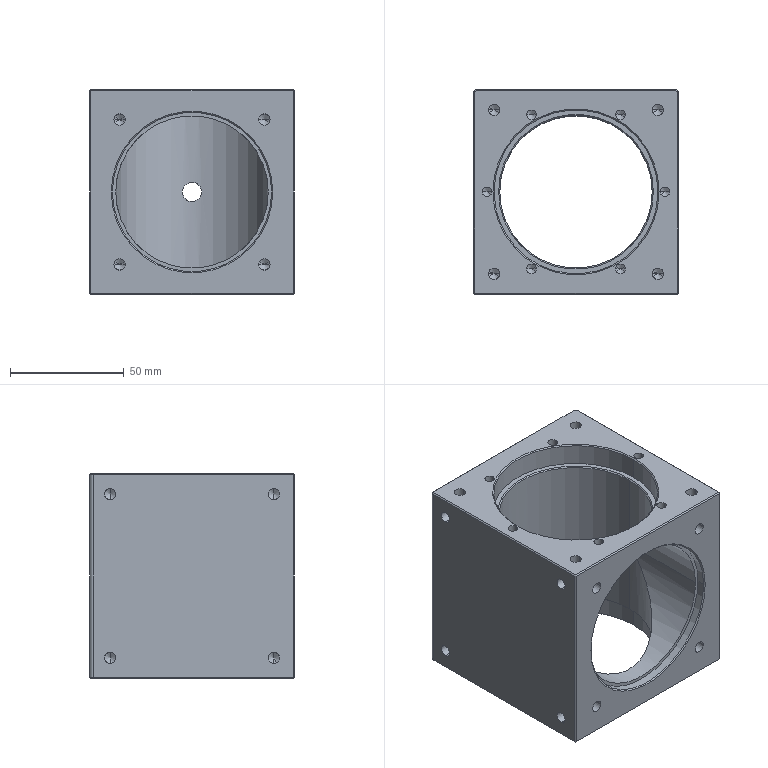NC program | NX | posted with a generic post | part box 90 x 90 x 90 mm
Whole program:
N10 G17 G21 G94 G90
(DRILLING_COPY_1_COPY_1_COPY , TOOL : D6A45)
N12 T07 M6
N14 G54
N16 G17 G0 G90 X19.55 Y-33.862 B0. C0. S5000 M3
N18 G43 Z30. H7
N20 G94 G81 G98 Z-1. F250. R3.
N22 X36. Y-36.
N24 X39.1 Y0.
N26 X36. Y36.
N28 X19.55 Y33.862
N30 X0. Y0.
N32 X-19.55 Y33.862
N34 X-36. Y36.
N36 X-39.1 Y0.
N38 X-36. Y-36.
N40 X-19.55 Y-33.862
N42 G80
N44 G0 X-19.55 Y-33.862 Z30.
N46 M5
(DRILLING_COPY_1_COPY_COPY_COPY_COPY_COPY_1 , TOOL : 5.0ZT)
N48 T15 M6
N50 G54
N52 G17 G0 G90 X36. Y-36. B0. C0. S2000 M3
N54 G43 Z30. H15
N56 G94 G83 G98 Z-12.002 F150. Q2. R3.
N58 X-36.
N60 Y36. Z-10.234
N62 X36.
N64 G80
N66 G0 X36. Y36. Z30.
N68 M5
(DRILLING_COPY_1_COPY_COPY_COPY_COPY_COPY_1_COPY , TOOL : 4.2ZT)
N70 T14 M6
N72 G54
N74 G17 G0 G90 X39.1 Y0. B0. C0. S2000 M3
N76 G43 Z30. H14
N78 G94 G83 G98 Z-15.262 F150. Q2. R3.
N80 X19.55 Y33.862
N82 X-19.55
N84 X-39.1 Y0.
N86 X-19.55 Y-33.862
N88 X19.55
N90 G80
N92 G0 X19.55 Y-33.862 Z30.
N94 M5
(DRILLING_COPY_1_COPY_COPY_COPY_COPY_COPY_COPY , TOOL : 9.0ZT)
N96 T09 M6
N98 G54
N100 G17 G0 G90 X0. Y0. B0. C0. S1200 M3
N102 G43 Z30. H9
N104 G94 G83 G98 Z-49.704 F150. Q2. R3.
N106 G80
N108 G0 X0. Y0. Z30.
N110 M5
(HOLE_MILLING_COPY_1 , TOOL : D10)
N112 T10 M6
N114 G54
N116 G17 G0 G90 X0. Y0. B0. C0. S9500 M3
N118 G43 Z30. H10
N120 Z0.5
N122 G94 G3 X1.25 Y-1.25 R1.25 F2200.
N124 X2.5 Y0. R1.25
N126 X2.5 Y0. Z-0.5 I-2.5 J0.
N128 X2.5 Y0. Z-1.5 I-2.5 J0.
N130 X2.5 Y0. Z-2.5 I-2.5 J0.
N132 X2.5 Y0. Z-3.5 I-2.5 J0.
N134 X2.5 Y0. Z-4.5 I-2.5 J0.
N136 X2.5 Y0. Z-5.5 I-2.5 J0.
N138 X2.5 Y0. Z-6.5 I-2.5 J0.
N140 X2.5 Y0. Z-7.5 I-2.5 J0.
N142 X2.5 Y0. Z-8.5 I-2.5 J0.
N144 X2.5 Y0. Z-9.5 I-2.5 J0.
N146 X-0.099 Y2.678 R2.68
N148 X-2.987 Y0.165 R2.819
N150 X-0.334 Y-3.217 R3.076
N152 X3.461 Y-0.383 R3.39
N154 X0.578 Y3.681 R3.568
N156 X-3.919 Y0.654 R3.881
N158 X-0.874 Y-4.126 R4.06
N160 X4.357 Y-0.976 R4.373
N162 X1.22 Y4.548 R4.551
N164 X-4.769 Y1.349 R4.865
N166 X-1.615 Y-4.943 R5.043
N168 X5.152 Y-1.769 R5.356
N170 X2.058 Y5.307 R5.534
N172 X-5.502 Y2.235 R5.847
N174 X-2.544 Y-5.635 R6.025
N176 X5.815 Y-2.744 R6.339
N178 X3.072 Y5.925 R6.517
N180 X-6.087 Y3.294 R6.83
N182 X-3.64 Y-6.172 R7.008
N184 X6.315 Y-3.882 R7.322
N186 X4.243 Y6.374 R7.5
N188 X-6.495 Y4.503 R7.813
N190 X-4.879 Y-6.526 R7.991
N192 X6.625 Y-5.156 R8.304
N194 X5.543 Y6.627 R8.482
N196 X-6.701 Y5.836 R8.796
N198 X-6.232 Y-6.673 R8.974
N200 X6.721 Y-6.539 R9.287
N202 X6.943 Y6.662 R9.465
N204 X-6.684 Y7.26 R9.778
N206 X-7.67 Y-6.592 R9.956
N208 X6.586 Y-7.997 R10.269
N210 X8.409 Y6.461 R10.447
N212 X-6.426 Y8.743 R10.761
N214 X-9.156 Y-6.268 R10.939
N216 X6.204 Y-9.495 R11.252
N218 X9.906 Y6.012 R11.43
N220 X-5.917 Y10.248 R11.743
N222 X-10.654 Y-5.691 R11.921
N224 X5.565 Y-10.997 R12.235
N226 X11.395 Y5.305 R12.413
N228 X-5.148 Y11.736 R12.726
N230 X-12.125 Y-4.854 R12.904
N232 X4.666 Y-12.462 R13.217
N234 X12.839 Y4.338 R13.395
N236 X-4.119 Y13.169 R13.708
N238 X-13.531 Y-3.758 R13.886
N240 X3.508 Y-13.852 R14.2
N242 X14.197 Y3.114 R14.378
N244 X-2.834 Y14.507 R14.691
N246 X-14.832 Y-2.408 R14.869
N248 X2.098 Y-15.127 R15.182
N250 X15.43 Y1.642 R15.36
N252 X-1.302 Y15.709 R15.673
N254 X-15.987 Y-0.816 R15.851
N256 X0.448 Y-16.248 R16.165
N258 X16.499 Y-0.066 R16.343
N260 X0.461 Y16.739 R16.656
N262 X-16.961 Y1.002 R16.834
N264 X-1.423 Y-17.178 R17.147
N266 X17.369 Y-1.989 R17.325
N268 X2.435 Y17.56 R17.638
N270 X-17.717 Y3.023 R17.816
N272 X-3.493 Y-17.881 R18.13
N274 X18.003 Y-4.102 R18.308
N276 X4.593 Y18.138 R18.621
N278 X-18.222 Y5.221 R18.799
N280 X-5.732 Y-18.326 R19.112
N282 X18.372 Y-6.377 R19.29
N284 X6.905 Y18.443 R19.603
N286 X-18.448 Y7.564 R19.781
N288 X-8.108 Y-18.484 R20.095
N290 X18.447 Y-8.778 R20.273
N292 X9.336 Y18.448 R20.586
N294 X-18.368 Y10.015 R20.764
N296 X-10.583 Y-18.331 R21.077
N298 X18.207 Y-11.269 R21.255
N300 X11.846 Y18.131 R21.568
N302 X-17.962 Y12.535 R21.746
N304 X-13.117 Y-17.847 R22.06
N306 X17.632 Y-13.807 R22.238
N308 X14.393 Y17.476 R22.551
N310 X-17.215 Y15.08 R22.729
N312 X-15.667 Y-17.018 R23.042
N314 X16.71 Y-16.348 R23.22
N316 X16.932 Y16.472 R23.533
N318 X-16.117 Y17.605 R23.711
N320 X-18.185 Y-15.837 R24.025
N322 X15.435 Y-18.845 R24.202
N324 X19.417 Y15.113 R24.516
N326 X-14.664 Y20.063 R24.694
N328 X-20.624 Y-14.3 R25.007
N330 X13.805 Y-21.251 R25.185
N332 X21.799 Y13.4 R25.498
N334 X-12.859 Y22.405 R25.676
N336 X-22.936 Y-12.412 R25.989
N338 X11.827 Y-23.518 R26.167
N340 X24.029 Y11.34 R26.481
N342 X-10.711 Y24.583 R26.659
N344 X-25.072 Y-10.183 R26.972
N346 X9.513 Y-25.596 R27.15
N348 X26.06 Y8.946 R27.463
N350 X-8.235 Y26.55 R27.641
N352 X-26.986 Y-7.631 R27.954
N354 X6.881 Y-27.44 R28.132
N356 X27.844 Y6.24 R28.446
N358 X-5.453 Y28.259 R28.624
N360 X-28.63 Y-4.778 R28.937
N362 X3.955 Y-29.003 R29.115
N364 X29.338 Y3.247 R29.428
N366 X-2.392 Y29.667 R29.606
N368 X-29.963 Y-1.653 R29.919
N370 X1.001 Y-30.316 R30.177
N372 X30.5 Y0. R30.328
N374 X0. Y30.5 R30.5
N376 X30.5 Y0. R-30.5
N378 X15.25 Y15.25 R15.25
N380 X0. Y0. R15.25
N382 G0 Z30.
N384 M5
(HOLE_MILLING_COPY_COPY_1 , TOOL : D16)
N386 T16 M6
N388 G54
N390 G17 G0 G90 X0. Y0. B0. C0. S8500 M3
N392 G43 Z30. H16
N394 Z-9.
N396 G94 G3 X1.5 Y-1.5 R1.5 F2200.
N398 X3. Y0. R1.5
N400 X3. Y0. Z-10. I-3. J0.
N402 X3. Y0. Z-11. I-3. J0.
N404 X3. Y0. Z-12. I-3. J0.
N406 X3. Y0. Z-13. I-3. J0.
N408 X3. Y0. Z-14. I-3. J0.
N410 X3. Y0. Z-15. I-3. J0.
N412 X3. Y0. Z-16. I-3. J0.
N414 X3. Y0. Z-17. I-3. J0.
N416 X3. Y0. Z-18. I-3. J0.
N418 X3. Y0. Z-19. I-3. J0.
N420 X3. Y0. Z-20. I-3. J0.
N422 X3. Y0. Z-21. I-3. J0.
N424 X3. Y0. Z-22. I-3. J0.
N426 X3. Y0. Z-23. I-3. J0.
N428 X3. Y0. Z-24. I-3. J0.
N430 X3. Y0. Z-25. I-3. J0.
N432 X3. Y0. Z-26. I-3. J0.
N434 X3. Y0. Z-27. I-3. J0.
N436 X0. Y-3. Z-27.75 R-3.
N438 X3.177 Y0.141 R3.177
N440 X0.073 Y3.496 R3.325
N442 X-3.738 Y0.186 R3.583
N444 X-0.167 Y-3.99 R3.9
N446 X4.23 Y-0.29 R4.08
N448 X0.282 Y4.481 R4.397
N450 X-4.718 Y0.415 R4.577
N452 X-0.417 Y-4.969 R4.894
N454 X5.203 Y-0.56 R5.074
N456 X0.573 Y5.453 R5.391
N458 X-5.684 Y0.726 R5.571
N460 X-0.749 Y-5.933 R5.888
N462 X6.16 Y-0.912 R6.068
N464 X0.946 Y6.407 R6.385
N466 X-6.63 Y1.119 R6.565
N468 X-1.163 Y-6.876 R6.881
N470 X7.094 Y-1.345 R7.062
N472 X1.4 Y7.338 R7.378
N474 X-7.551 Y1.592 R7.558
N476 X-1.656 Y-7.793 R7.875
N478 X8.001 Y-1.858 R8.055
N480 X1.933 Y8.24 R8.372
N482 X-8.443 Y2.143 R8.552
N484 X-2.228 Y-8.679 R8.868
N486 X8.876 Y-2.448 R9.049
N488 X2.543 Y9.108 R9.365
N490 X-9.3 Y2.772 R9.545
N492 X-2.877 Y-9.529 R9.862
N494 X9.714 Y-3.115 R10.042
N496 X3.229 Y9.939 R10.359
N498 X-10.117 Y3.476 R10.539
N500 X-3.6 Y-10.338 R10.855
N502 X10.509 Y-3.855 R11.036
N504 X3.989 Y10.726 R11.352
N506 X-10.89 Y4.253 R11.532
N508 X-4.395 Y-11.102 R11.849
N510 X11.259 Y-4.667 R12.029
N512 X4.819 Y11.465 R12.346
N514 X-11.614 Y5.099 R12.526
N516 X-5.26 Y-11.815 R12.842
N518 X11.956 Y-5.548 R13.022
N520 X5.718 Y12.152 R13.339
N522 X-12.285 Y6.014 R13.519
N524 X-6.192 Y-12.474 R13.836
N526 X12.599 Y-6.495 R14.016
N528 X6.682 Y12.782 R14.332
N530 X-12.898 Y6.992 R14.513
N532 X-7.188 Y-13.074 R14.829
N534 X13.181 Y-7.505 R15.009
N536 X7.708 Y13.351 R15.326
N538 X-13.449 Y8.032 R15.506
N540 X-8.244 Y-13.612 R15.822
N542 X13.7 Y-8.573 R16.003
N544 X8.793 Y13.855 R16.319
N546 X-13.934 Y9.129 R16.499
N548 X-9.356 Y-14.082 R16.816
N550 X14.15 Y-9.698 R16.996
N552 X9.932 Y14.291 R17.312
N554 X-14.349 Y10.28 R17.493
N556 X-10.521 Y-14.481 R17.809
N558 X14.529 Y-10.874 R17.989
N560 X11.123 Y14.653 R18.306
N562 X-14.691 Y11.481 R18.486
N564 X-11.736 Y-14.807 R18.803
N566 X14.833 Y-12.098 R18.983
N568 X12.36 Y14.94 R19.299
N570 X-14.956 Y12.727 R19.479
N572 X-12.994 Y-15.054 R19.796
N574 X15.059 Y-13.366 R19.976
N576 X13.639 Y15.148 R20.293
N578 X-15.141 Y14.014 R20.473
N580 X-14.293 Y-15.221 R20.789
N582 X15.203 Y-14.672 R20.97
N584 X14.956 Y15.273 R21.286
N586 X-15.243 Y15.338 R21.466
N588 X-15.628 Y-15.304 R21.783
N590 X15.262 Y-16.013 R21.963
N592 X16.307 Y15.313 R22.279
N594 X-15.26 Y16.695 R22.46
N596 X-16.993 Y-15.301 R22.776
N598 X15.235 Y-17.383 R22.956
N600 X17.686 Y15.266 R23.273
N602 X-15.189 Y18.078 R23.453
N604 X-18.384 Y-15.209 R23.769
N606 X15.119 Y-18.778 R23.95
N608 X19.088 Y15.129 R24.266
N610 X-15.027 Y19.483 R24.446
N612 X-19.796 Y-15.026 R24.763
N614 X15.149 Y-20.116 R25.023
N616 X20.509 Y14.9 R25.179
N618 X-14.9 Y20.509 R25.35
N620 X20.509 Y14.9 R-25.35
N622 X2.804 Y17.704 R12.675
N624 X0. Y0. R12.675
N626 X1.5 Y-1.5 R1.5
N628 X3. Y0. R1.5
N630 X3. Y0. Z-28.75 I-3. J0.
N632 X3. Y0. Z-29.75 I-3. J0.
N634 X3. Y0. Z-30.75 I-3. J0.
N636 X3. Y0. Z-31.75 I-3. J0.
N638 X3. Y0. Z-32.75 I-3. J0.
N640 X3. Y0. Z-33.75 I-3. J0.
N642 X3. Y0. Z-34.75 I-3. J0.
N644 X3. Y0. Z-35.75 I-3. J0.
N646 X3. Y0. Z-36.75 I-3. J0.
N648 X3. Y0. Z-37.75 I-3. J0.
N650 X3. Y0. Z-38.75 I-3. J0.
N652 X3. Y0. Z-39.75 I-3. J0.
N654 X3. Y0. Z-40.75 I-3. J0.
N656 X3. Y0. Z-41.75 I-3. J0.
N658 X3. Y0. Z-42.75 I-3. J0.
N660 X3. Y0. Z-43.75 I-3. J0.
N662 X3. Y0. Z-44.75 I-3. J0.
N664 X3. Y0. Z-45.75 I-3. J0.
N666 X0. Y-3. Z-46.5 R-3.
N668 X3.177 Y0.141 R3.177
N670 X0.073 Y3.496 R3.325
N672 X-3.738 Y0.186 R3.583
N674 X-0.167 Y-3.99 R3.9
N676 X4.23 Y-0.29 R4.08
N678 X0.282 Y4.481 R4.397
N680 X-4.718 Y0.415 R4.577
N682 X-0.417 Y-4.969 R4.894
N684 X5.203 Y-0.56 R5.074
N686 X0.573 Y5.453 R5.391
N688 X-5.684 Y0.726 R5.571
N690 X-0.749 Y-5.933 R5.888
N692 X6.16 Y-0.912 R6.068
N694 X0.946 Y6.407 R6.385
N696 X-6.63 Y1.119 R6.565
N698 X-1.163 Y-6.876 R6.881
N700 X7.094 Y-1.345 R7.062
N702 X1.4 Y7.338 R7.378
N704 X-7.551 Y1.592 R7.558
N706 X-1.656 Y-7.793 R7.875
N708 X8.001 Y-1.858 R8.055
N710 X1.933 Y8.24 R8.372
N712 X-8.443 Y2.143 R8.552
N714 X-2.228 Y-8.679 R8.868
N716 X8.876 Y-2.448 R9.049
N718 X2.543 Y9.108 R9.365
N720 X-9.3 Y2.772 R9.545
N722 X-2.877 Y-9.529 R9.862
N724 X9.714 Y-3.115 R10.042
N726 X3.229 Y9.939 R10.359
N728 X-10.117 Y3.476 R10.539
N730 X-3.6 Y-10.338 R10.855
N732 X10.509 Y-3.855 R11.036
N734 X3.989 Y10.726 R11.352
N736 X-10.89 Y4.253 R11.532
N738 X-4.395 Y-11.102 R11.849
N740 X11.259 Y-4.667 R12.029
N742 X4.819 Y11.465 R12.346
N744 X-11.614 Y5.099 R12.526
N746 X-5.26 Y-11.815 R12.842
N748 X11.956 Y-5.548 R13.022
N750 X5.718 Y12.152 R13.339
N752 X-12.285 Y6.014 R13.519
N754 X-6.192 Y-12.474 R13.836
N756 X12.599 Y-6.495 R14.016
N758 X6.682 Y12.782 R14.332
N760 X-12.898 Y6.992 R14.513
N762 X-7.188 Y-13.074 R14.829
N764 X13.181 Y-7.505 R15.009
N766 X7.708 Y13.351 R15.326
N768 X-13.449 Y8.032 R15.506
N770 X-8.244 Y-13.612 R15.822
N772 X13.7 Y-8.573 R16.003
N774 X8.793 Y13.855 R16.319
N776 X-13.934 Y9.129 R16.499
N778 X-9.356 Y-14.082 R16.816
N780 X14.15 Y-9.698 R16.996
N782 X9.932 Y14.291 R17.312
N784 X-14.349 Y10.28 R17.493
N786 X-10.521 Y-14.481 R17.809
N788 X14.529 Y-10.874 R17.989
N790 X11.123 Y14.653 R18.306
N792 X-14.691 Y11.481 R18.486
N794 X-11.736 Y-14.807 R18.803
N796 X14.833 Y-12.098 R18.983
N798 X12.36 Y14.94 R19.299
N800 X-14.956 Y12.727 R19.479
N802 X-12.994 Y-15.054 R19.796
N804 X15.059 Y-13.366 R19.976
N806 X13.639 Y15.148 R20.293
N808 X-15.141 Y14.014 R20.473
N810 X-14.293 Y-15.221 R20.789
N812 X15.203 Y-14.672 R20.97
N814 X14.956 Y15.273 R21.286
N816 X-15.243 Y15.338 R21.466
N818 X-15.628 Y-15.304 R21.783
N820 X15.262 Y-16.013 R21.963
N822 X16.307 Y15.313 R22.279
N824 X-15.26 Y16.695 R22.46
N826 X-16.993 Y-15.301 R22.776
N828 X15.235 Y-17.383 R22.956
N830 X17.686 Y15.266 R23.273
N832 X-15.189 Y18.078 R23.453
N834 X-18.384 Y-15.209 R23.769
N836 X15.119 Y-18.778 R23.95
N838 X19.088 Y15.129 R24.266
N840 X-15.027 Y19.483 R24.446
N842 X-19.796 Y-15.026 R24.763
N844 X15.149 Y-20.116 R25.023
N846 X20.509 Y14.9 R25.179
N848 X-14.9 Y20.509 R25.35
N850 X20.509 Y14.9 R-25.35
N852 X2.804 Y17.704 R12.675
N854 X0. Y0. R12.675
N856 G0 Z30.
N858 M5
(HOLE_MILLING_COPY_COPY_COPY , TOOL : D12JING)
N860 T12 M6
N862 G54
N864 G17 G0 G90 X23.779 Y-3.247 B0. C0. S8000 M3
N866 G43 Z30. H12
N868 Z-27.75
N870 G94 G3 X27.5 Y0. R3.277 F1000.
N872 X0. Y27.5 R27.5
N874 X27.5 Y0. R-27.5
N876 X23.779 Y3.247 R3.277
N878 G0 Y-3.247 Z-46.5
N880 G3 X27.5 Y0. R3.277
N882 X0. Y27.5 R27.5
N884 X27.5 Y0. R-27.5
N886 X23.779 Y3.247 R3.277
N888 G0 Z30.
N890 M5
(ZLEVEL_PROFILE_1_COPY_1_COPY_COPY , TOOL : D6A45)
N892 T07 M6
N894 G54
N896 G17 G0 G90 X-36.315 Y36.132 B0. C0. S9500 M3
N898 G43 Z30. H7
N900 Z0.
N902 G94 G1 Z-1. F1000.
N904 X-37.241 Y36.52
N906 G3 X-37.541 Y36. R0.6
N908 X-36. Y34.459 R1.541
N910 X-37.541 Y36. R-1.541
N912 X-37.241 Y35.48 R0.6
N914 G1 X-36.315 Y35.868
N916 Z0.
N918 G0 Z30.
N920 X36.132 Y36.315
N922 Z0.
N924 G1 Z-1.
N926 X36.52 Y37.241
N928 G3 X36. Y37.541 R0.6
N930 X34.459 Y36. R1.541
N932 X36. Y37.541 R-1.541
N934 X35.48 Y37.241 R0.6
N936 G1 X35.868 Y36.315
N938 Z0.
N940 G0 Z30.
N942 X-19.55 Y35.003
N944 Z1.
N946 G1 Z-1.
N948 G3 X-20.691 Y33.862 R1.141
N950 X-19.55 Y35.003 R-1.141
N952 X-20.07 Y34.703 R0.6
N954 G1 Z0.
N956 G0 Z30.
N958 X19.55 Y-35.003
N960 Z1.
N962 G1 Z-1.
N964 G3 X20.691 Y-33.862 R1.141
N966 X19.55 Y-35.003 R-1.141
N968 X20.07 Y-34.703 R0.6
N970 G1 Z0.
N972 G0 Z30.
N974 X40.241 Y0.
N976 Z1.
N978 G1 Z-1.
N980 G3 X39.1 Y1.141 R1.141
N982 X40.241 Y0. R-1.141
N984 X39.941 Y0.52 R0.6
N986 G1 Z0.
N988 G0 Z30.
N990 X36.315 Y-36.132
N992 Z0.
N994 G1 Z-1.
N996 X37.241 Y-36.52
N998 G3 X37.541 Y-36. R0.6
N1000 X36. Y-34.459 R1.541
N1002 X37.541 Y-36. R-1.541
N1004 X37.241 Y-35.48 R0.6
N1006 G1 X36.315 Y-35.868
N1008 Z0.
N1010 G0 Z30.
N1012 X34.325 Y-1.048
N1014 Z0.
N1016 G1 Z-1.
N1018 X35.241 Y-0.52
N1020 G3 X35.541 Y0. R0.6
N1022 G1 Y0.008
N1024 G3 X-0.008 Y35.541 R35.541
N1026 X35.541 Y0. R-35.541
N1028 X35.241 Y0.52 R0.6
N1030 G1 X34.325 Y1.048
N1032 Z0.
N1034 G0 Z30.
N1036 X-40.241 Y0.
N1038 Z1.
N1040 G1 Z-1.
N1042 Y-0.003
N1044 G3 X-39.097 Y-1.141 R1.141
N1046 X-40.241 Y0. R-1.141
N1048 X-39.941 Y-0.52 R0.6
N1050 G1 Z0.
N1052 G0 Z30.
N1054 X-36.315 Y-35.868
N1056 Z0.
N1058 G1 Z-1.
N1060 X-37.241 Y-35.48
N1062 G3 X-37.541 Y-36. R0.6
N1064 G1 Y-36.003
N1066 G3 X-35.997 Y-37.541 R1.541
N1068 X-37.541 Y-36. R-1.541
N1070 X-37.241 Y-36.52 R0.6
N1072 G1 X-36.315 Y-36.132
N1074 Z0.
N1076 G0 Z30.
N1078 X19.55 Y35.003
N1080 Z1.
N1082 G1 Z-1.
N1084 G3 X18.409 Y33.862 R1.141
N1086 X19.55 Y35.003 R-1.141
N1088 X19.03 Y34.703 R0.6
N1090 G1 Z0.
N1092 G0 Z30.
N1094 X-19.55 Y-35.003
N1096 Z1.
N1098 G1 Z-1.
N1100 G3 X-18.409 Y-33.862 R1.141
N1102 X-19.55 Y-35.003 R-1.141
N1104 X-19.03 Y-34.703 R0.6
N1106 G1 Z0.
N1108 G0 Z30.
N1110 X45.421 Y-46.453
N1112 Z0.
N1114 G1 Z-1.
N1116 X45.02 Y-45.759
N1118 G3 X44.501 Y-45.459 R0.6
N1120 G1 X-44.501
N1122 G2 X-45.459 Y-44.501 R0.958
N1124 G1 Y43.5
N1126 G2 X-43.5 Y45.459 R1.959
N1128 G1 X43.5
N1130 G2 X45.459 Y43.5 R1.959
N1132 G1 Y-44.501
N1134 G2 X44.501 Y-45.459 R0.958
N1136 G3 X43.981 Y-45.759 R0.6
N1138 G1 X43.462 Y-46.659
N1140 Z0.
N1142 G0 Z30.
N1144 M5
N1146 M2